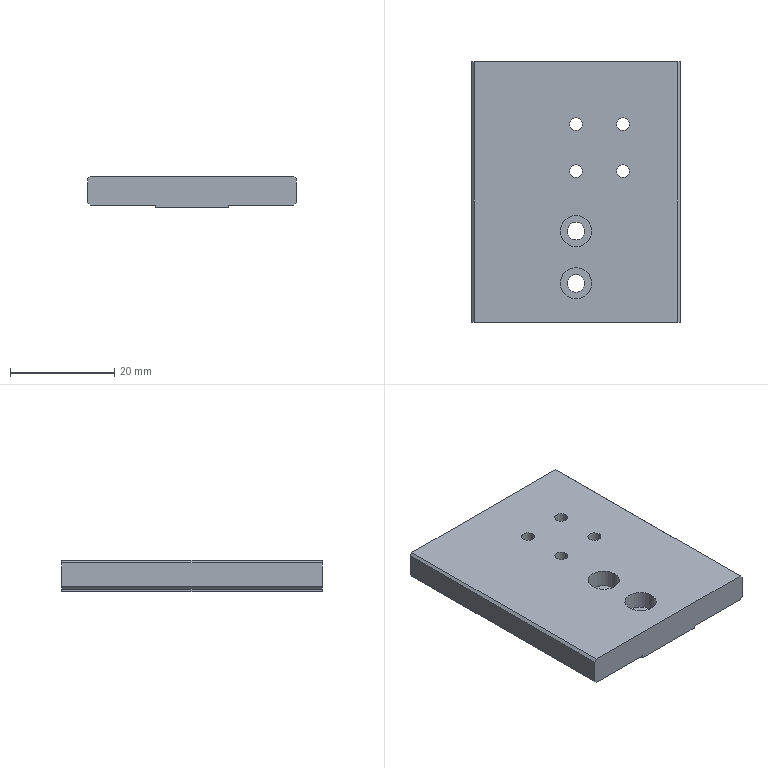Part | SolidWorks | features HoleWzd 2, Chamfer 1, Extrusion 1 | 1 solid | 32 faces | box 40 x 50 x 6 mm | volume 10973 mm3 | cylinder 16 | plane 16 | commonest cylinder face diameters 2.5 x8 3.4 x4 6 x4
STEP:
#1=CARTESIAN_POINT('',(18.75,13.,-6.));
#2=VERTEX_POINT('',#1);
#3=CARTESIAN_POINT('',(21.25,13.,-6.));
#4=VERTEX_POINT('',#3);
#5=CARTESIAN_POINT('',(20.,13.,-6.));
#6=DIRECTION('',(0.,0.,1.));
#7=DIRECTION('',(1.,0.,0.));
#8=AXIS2_PLACEMENT_3D('',#5,#6,#7);
#9=CIRCLE('',#8,1.25);
#10=EDGE_CURVE('',#2,#4,#9,.T.);
#11=ORIENTED_EDGE('',*,*,#10,.F.);
#12=CARTESIAN_POINT('',(18.75,13.,0.));
#13=VERTEX_POINT('',#12);
#14=CARTESIAN_POINT('',(18.75,13.,0.));
#15=DIRECTION('',(0.,0.,1.));
#16=VECTOR('',#15,1000.);
#17=LINE('',#14,#16);
#18=EDGE_CURVE('',#2,#13,#17,.T.);
#19=ORIENTED_EDGE('',*,*,#18,.T.);
#20=CARTESIAN_POINT('',(21.25,13.,0.));
#21=VERTEX_POINT('',#20);
#22=CARTESIAN_POINT('',(20.,13.,0.));
#23=DIRECTION('',(0.,0.,1.));
#24=DIRECTION('',(1.,0.,0.));
#25=AXIS2_PLACEMENT_3D('',#22,#23,#24);
#26=CIRCLE('',#25,1.25);
#27=EDGE_CURVE('',#13,#21,#26,.T.);
#28=ORIENTED_EDGE('',*,*,#27,.T.);
#29=CARTESIAN_POINT('',(21.25,13.,0.));
#30=DIRECTION('',(0.,0.,1.));
#31=VECTOR('',#30,1000.);
#32=LINE('',#29,#31);
#33=EDGE_CURVE('',#4,#21,#32,.T.);
#34=ORIENTED_EDGE('',*,*,#33,.F.);
#35=EDGE_LOOP('',(#11,#19,#28,#34));
#36=FACE_OUTER_BOUND('',#35,.T.);
#37=CARTESIAN_POINT('',(20.,13.,0.));
#38=DIRECTION('',(0.,0.,1.));
#39=DIRECTION('',(1.,0.,0.));
#40=AXIS2_PLACEMENT_3D('',#37,#38,#39);
#41=CYLINDRICAL_SURFACE('',#40,1.25);
#42=ADVANCED_FACE('',(#36),#41,.F.);
#43=CARTESIAN_POINT('',(27.75,13.,-5.5));
#44=VERTEX_POINT('',#43);
#45=CARTESIAN_POINT('',(30.25,13.,-5.5));
#46=VERTEX_POINT('',#45);
#47=CARTESIAN_POINT('',(29.,13.,-5.5));
#48=DIRECTION('',(0.,0.,1.));
#49=DIRECTION('',(1.,0.,0.));
#50=AXIS2_PLACEMENT_3D('',#47,#48,#49);
#51=CIRCLE('',#50,1.25);
#52=EDGE_CURVE('',#44,#46,#51,.T.);
#53=ORIENTED_EDGE('',*,*,#52,.F.);
#54=CARTESIAN_POINT('',(27.75,13.,0.));
#55=VERTEX_POINT('',#54);
#56=CARTESIAN_POINT('',(27.75,13.,0.));
#57=DIRECTION('',(0.,0.,1.));
#58=VECTOR('',#57,1000.);
#59=LINE('',#56,#58);
#60=EDGE_CURVE('',#44,#55,#59,.T.);
#61=ORIENTED_EDGE('',*,*,#60,.T.);
#62=CARTESIAN_POINT('',(30.25,13.,0.));
#63=VERTEX_POINT('',#62);
#64=CARTESIAN_POINT('',(29.,13.,0.));
#65=DIRECTION('',(0.,0.,1.));
#66=DIRECTION('',(1.,0.,0.));
#67=AXIS2_PLACEMENT_3D('',#64,#65,#66);
#68=CIRCLE('',#67,1.25);
#69=EDGE_CURVE('',#55,#63,#68,.T.);
#70=ORIENTED_EDGE('',*,*,#69,.T.);
#71=CARTESIAN_POINT('',(30.25,13.,0.));
#72=DIRECTION('',(0.,0.,1.));
#73=VECTOR('',#72,1000.);
#74=LINE('',#71,#73);
#75=EDGE_CURVE('',#46,#63,#74,.T.);
#76=ORIENTED_EDGE('',*,*,#75,.F.);
#77=EDGE_LOOP('',(#53,#61,#70,#76));
#78=FACE_OUTER_BOUND('',#77,.T.);
#79=CARTESIAN_POINT('',(29.,13.,0.));
#80=DIRECTION('',(0.,0.,1.));
#81=DIRECTION('',(1.,0.,0.));
#82=AXIS2_PLACEMENT_3D('',#79,#80,#81);
#83=CYLINDRICAL_SURFACE('',#82,1.25);
#84=ADVANCED_FACE('',(#78),#83,.F.);
#85=CARTESIAN_POINT('',(18.75,4.,-6.));
#86=VERTEX_POINT('',#85);
#87=CARTESIAN_POINT('',(21.25,4.,-6.));
#88=VERTEX_POINT('',#87);
#89=CARTESIAN_POINT('',(20.,4.,-6.));
#90=DIRECTION('',(0.,0.,1.));
#91=DIRECTION('',(1.,0.,0.));
#92=AXIS2_PLACEMENT_3D('',#89,#90,#91);
#93=CIRCLE('',#92,1.25);
#94=EDGE_CURVE('',#86,#88,#93,.T.);
#95=ORIENTED_EDGE('',*,*,#94,.F.);
#96=CARTESIAN_POINT('',(18.75,4.,0.));
#97=VERTEX_POINT('',#96);
#98=CARTESIAN_POINT('',(18.75,4.,0.));
#99=DIRECTION('',(0.,0.,1.));
#100=VECTOR('',#99,1000.);
#101=LINE('',#98,#100);
#102=EDGE_CURVE('',#86,#97,#101,.T.);
#103=ORIENTED_EDGE('',*,*,#102,.T.);
#104=CARTESIAN_POINT('',(21.25,4.,0.));
#105=VERTEX_POINT('',#104);
#106=CARTESIAN_POINT('',(20.,4.,0.));
#107=DIRECTION('',(0.,0.,1.));
#108=DIRECTION('',(1.,0.,0.));
#109=AXIS2_PLACEMENT_3D('',#106,#107,#108);
#110=CIRCLE('',#109,1.25);
#111=EDGE_CURVE('',#97,#105,#110,.T.);
#112=ORIENTED_EDGE('',*,*,#111,.T.);
#113=CARTESIAN_POINT('',(21.25,4.,0.));
#114=DIRECTION('',(0.,0.,1.));
#115=VECTOR('',#114,1000.);
#116=LINE('',#113,#115);
#117=EDGE_CURVE('',#88,#105,#116,.T.);
#118=ORIENTED_EDGE('',*,*,#117,.F.);
#119=EDGE_LOOP('',(#95,#103,#112,#118));
#120=FACE_OUTER_BOUND('',#119,.T.);
#121=CARTESIAN_POINT('',(20.,4.,0.));
#122=DIRECTION('',(0.,0.,1.));
#123=DIRECTION('',(1.,0.,0.));
#124=AXIS2_PLACEMENT_3D('',#121,#122,#123);
#125=CYLINDRICAL_SURFACE('',#124,1.25);
#126=ADVANCED_FACE('',(#120),#125,.F.);
#127=CARTESIAN_POINT('',(27.75,4.,-5.5));
#128=VERTEX_POINT('',#127);
#129=CARTESIAN_POINT('',(30.25,4.,-5.5));
#130=VERTEX_POINT('',#129);
#131=CARTESIAN_POINT('',(29.,4.,-5.5));
#132=DIRECTION('',(0.,0.,1.));
#133=DIRECTION('',(1.,0.,0.));
#134=AXIS2_PLACEMENT_3D('',#131,#132,#133);
#135=CIRCLE('',#134,1.25);
#136=EDGE_CURVE('',#128,#130,#135,.T.);
#137=ORIENTED_EDGE('',*,*,#136,.F.);
#138=CARTESIAN_POINT('',(27.75,4.,0.));
#139=VERTEX_POINT('',#138);
#140=CARTESIAN_POINT('',(27.75,4.,0.));
#141=DIRECTION('',(0.,0.,1.));
#142=VECTOR('',#141,1000.);
#143=LINE('',#140,#142);
#144=EDGE_CURVE('',#128,#139,#143,.T.);
#145=ORIENTED_EDGE('',*,*,#144,.T.);
#146=CARTESIAN_POINT('',(30.25,4.,0.));
#147=VERTEX_POINT('',#146);
#148=CARTESIAN_POINT('',(29.,4.,0.));
#149=DIRECTION('',(0.,0.,1.));
#150=DIRECTION('',(1.,0.,0.));
#151=AXIS2_PLACEMENT_3D('',#148,#149,#150);
#152=CIRCLE('',#151,1.25);
#153=EDGE_CURVE('',#139,#147,#152,.T.);
#154=ORIENTED_EDGE('',*,*,#153,.T.);
#155=CARTESIAN_POINT('',(30.25,4.,0.));
#156=DIRECTION('',(0.,0.,1.));
#157=VECTOR('',#156,1000.);
#158=LINE('',#155,#157);
#159=EDGE_CURVE('',#130,#147,#158,.T.);
#160=ORIENTED_EDGE('',*,*,#159,.F.);
#161=EDGE_LOOP('',(#137,#145,#154,#160));
#162=FACE_OUTER_BOUND('',#161,.T.);
#163=CARTESIAN_POINT('',(29.,4.,0.));
#164=DIRECTION('',(0.,0.,1.));
#165=DIRECTION('',(1.,0.,0.));
#166=AXIS2_PLACEMENT_3D('',#163,#164,#165);
#167=CYLINDRICAL_SURFACE('',#166,1.25);
#168=ADVANCED_FACE('',(#162),#167,.F.);
#169=CARTESIAN_POINT('',(17.,-7.5,-3.4));
#170=VERTEX_POINT('',#169);
#171=CARTESIAN_POINT('',(23.,-7.5,-3.4));
#172=VERTEX_POINT('',#171);
#173=CARTESIAN_POINT('',(20.,-7.5,-3.4));
#174=DIRECTION('',(0.,0.,1.));
#175=DIRECTION('',(1.,0.,0.));
#176=AXIS2_PLACEMENT_3D('',#173,#174,#175);
#177=CIRCLE('',#176,3.);
#178=EDGE_CURVE('',#170,#172,#177,.T.);
#179=ORIENTED_EDGE('',*,*,#178,.F.);
#180=CARTESIAN_POINT('',(17.,-7.5,0.));
#181=VERTEX_POINT('',#180);
#182=CARTESIAN_POINT('',(17.,-7.5,0.));
#183=DIRECTION('',(0.,0.,1.));
#184=VECTOR('',#183,1000.);
#185=LINE('',#182,#184);
#186=EDGE_CURVE('',#170,#181,#185,.T.);
#187=ORIENTED_EDGE('',*,*,#186,.T.);
#188=CARTESIAN_POINT('',(23.,-7.5,0.));
#189=VERTEX_POINT('',#188);
#190=CARTESIAN_POINT('',(20.,-7.5,0.));
#191=DIRECTION('',(0.,0.,1.));
#192=DIRECTION('',(1.,0.,0.));
#193=AXIS2_PLACEMENT_3D('',#190,#191,#192);
#194=CIRCLE('',#193,3.);
#195=EDGE_CURVE('',#181,#189,#194,.T.);
#196=ORIENTED_EDGE('',*,*,#195,.T.);
#197=CARTESIAN_POINT('',(23.,-7.5,0.));
#198=DIRECTION('',(0.,0.,1.));
#199=VECTOR('',#198,1000.);
#200=LINE('',#197,#199);
#201=EDGE_CURVE('',#172,#189,#200,.T.);
#202=ORIENTED_EDGE('',*,*,#201,.F.);
#203=EDGE_LOOP('',(#179,#187,#196,#202));
#204=FACE_OUTER_BOUND('',#203,.T.);
#205=CARTESIAN_POINT('',(20.,-7.5,0.));
#206=DIRECTION('',(0.,0.,1.));
#207=DIRECTION('',(1.,0.,0.));
#208=AXIS2_PLACEMENT_3D('',#205,#206,#207);
#209=CYLINDRICAL_SURFACE('',#208,3.);
#210=ADVANCED_FACE('',(#204),#209,.F.);
#211=CARTESIAN_POINT('',(18.3,-7.5,-6.));
#212=VERTEX_POINT('',#211);
#213=CARTESIAN_POINT('',(21.7,-7.5,-6.));
#214=VERTEX_POINT('',#213);
#215=CARTESIAN_POINT('',(20.,-7.5,-6.));
#216=DIRECTION('',(0.,0.,1.));
#217=DIRECTION('',(1.,0.,0.));
#218=AXIS2_PLACEMENT_3D('',#215,#216,#217);
#219=CIRCLE('',#218,1.7);
#220=EDGE_CURVE('',#212,#214,#219,.T.);
#221=ORIENTED_EDGE('',*,*,#220,.F.);
#222=CARTESIAN_POINT('',(18.3,-7.5,-3.4));
#223=VERTEX_POINT('',#222);
#224=CARTESIAN_POINT('',(18.3,-7.5,0.));
#225=DIRECTION('',(0.,0.,1.));
#226=VECTOR('',#225,1000.);
#227=LINE('',#224,#226);
#228=EDGE_CURVE('',#212,#223,#227,.T.);
#229=ORIENTED_EDGE('',*,*,#228,.T.);
#230=CARTESIAN_POINT('',(21.7,-7.5,-3.4));
#231=VERTEX_POINT('',#230);
#232=CARTESIAN_POINT('',(20.,-7.5,-3.4));
#233=DIRECTION('',(0.,0.,1.));
#234=DIRECTION('',(1.,0.,0.));
#235=AXIS2_PLACEMENT_3D('',#232,#233,#234);
#236=CIRCLE('',#235,1.7);
#237=EDGE_CURVE('',#223,#231,#236,.T.);
#238=ORIENTED_EDGE('',*,*,#237,.T.);
#239=CARTESIAN_POINT('',(21.7,-7.5,0.));
#240=DIRECTION('',(0.,0.,1.));
#241=VECTOR('',#240,1000.);
#242=LINE('',#239,#241);
#243=EDGE_CURVE('',#214,#231,#242,.T.);
#244=ORIENTED_EDGE('',*,*,#243,.F.);
#245=EDGE_LOOP('',(#221,#229,#238,#244));
#246=FACE_OUTER_BOUND('',#245,.T.);
#247=CARTESIAN_POINT('',(20.,-7.5,0.));
#248=DIRECTION('',(0.,0.,1.));
#249=DIRECTION('',(1.,0.,0.));
#250=AXIS2_PLACEMENT_3D('',#247,#248,#249);
#251=CYLINDRICAL_SURFACE('',#250,1.7);
#252=ADVANCED_FACE('',(#246),#251,.F.);
#253=CARTESIAN_POINT('',(17.,-17.5,-3.4));
#254=VERTEX_POINT('',#253);
#255=CARTESIAN_POINT('',(23.,-17.5,-3.4));
#256=VERTEX_POINT('',#255);
#257=CARTESIAN_POINT('',(20.,-17.5,-3.4));
#258=DIRECTION('',(0.,0.,1.));
#259=DIRECTION('',(1.,0.,0.));
#260=AXIS2_PLACEMENT_3D('',#257,#258,#259);
#261=CIRCLE('',#260,3.);
#262=EDGE_CURVE('',#254,#256,#261,.T.);
#263=ORIENTED_EDGE('',*,*,#262,.F.);
#264=CARTESIAN_POINT('',(17.,-17.5,0.));
#265=VERTEX_POINT('',#264);
#266=CARTESIAN_POINT('',(17.,-17.5,0.));
#267=DIRECTION('',(0.,0.,1.));
#268=VECTOR('',#267,1000.);
#269=LINE('',#266,#268);
#270=EDGE_CURVE('',#254,#265,#269,.T.);
#271=ORIENTED_EDGE('',*,*,#270,.T.);
#272=CARTESIAN_POINT('',(23.,-17.5,0.));
#273=VERTEX_POINT('',#272);
#274=CARTESIAN_POINT('',(20.,-17.5,0.));
#275=DIRECTION('',(0.,0.,1.));
#276=DIRECTION('',(1.,0.,0.));
#277=AXIS2_PLACEMENT_3D('',#274,#275,#276);
#278=CIRCLE('',#277,3.);
#279=EDGE_CURVE('',#265,#273,#278,.T.);
#280=ORIENTED_EDGE('',*,*,#279,.T.);
#281=CARTESIAN_POINT('',(23.,-17.5,0.));
#282=DIRECTION('',(0.,0.,1.));
#283=VECTOR('',#282,1000.);
#284=LINE('',#281,#283);
#285=EDGE_CURVE('',#256,#273,#284,.T.);
#286=ORIENTED_EDGE('',*,*,#285,.F.);
#287=EDGE_LOOP('',(#263,#271,#280,#286));
#288=FACE_OUTER_BOUND('',#287,.T.);
#289=CARTESIAN_POINT('',(20.,-17.5,0.));
#290=DIRECTION('',(0.,0.,1.));
#291=DIRECTION('',(1.,0.,0.));
#292=AXIS2_PLACEMENT_3D('',#289,#290,#291);
#293=CYLINDRICAL_SURFACE('',#292,3.);
#294=ADVANCED_FACE('',(#288),#293,.F.);
#295=CARTESIAN_POINT('',(18.3,-17.5,-6.));
#296=VERTEX_POINT('',#295);
#297=CARTESIAN_POINT('',(21.7,-17.5,-6.));
#298=VERTEX_POINT('',#297);
#299=CARTESIAN_POINT('',(20.,-17.5,-6.));
#300=DIRECTION('',(0.,0.,1.));
#301=DIRECTION('',(1.,0.,0.));
#302=AXIS2_PLACEMENT_3D('',#299,#300,#301);
#303=CIRCLE('',#302,1.7);
#304=EDGE_CURVE('',#296,#298,#303,.T.);
#305=ORIENTED_EDGE('',*,*,#304,.F.);
#306=CARTESIAN_POINT('',(18.3,-17.5,-3.4));
#307=VERTEX_POINT('',#306);
#308=CARTESIAN_POINT('',(18.3,-17.5,0.));
#309=DIRECTION('',(0.,0.,1.));
#310=VECTOR('',#309,1000.);
#311=LINE('',#308,#310);
#312=EDGE_CURVE('',#296,#307,#311,.T.);
#313=ORIENTED_EDGE('',*,*,#312,.T.);
#314=CARTESIAN_POINT('',(21.7,-17.5,-3.4));
#315=VERTEX_POINT('',#314);
#316=CARTESIAN_POINT('',(20.,-17.5,-3.4));
#317=DIRECTION('',(0.,0.,1.));
#318=DIRECTION('',(1.,0.,0.));
#319=AXIS2_PLACEMENT_3D('',#316,#317,#318);
#320=CIRCLE('',#319,1.7);
#321=EDGE_CURVE('',#307,#315,#320,.T.);
#322=ORIENTED_EDGE('',*,*,#321,.T.);
#323=CARTESIAN_POINT('',(21.7,-17.5,0.));
#324=DIRECTION('',(0.,0.,1.));
#325=VECTOR('',#324,1000.);
#326=LINE('',#323,#325);
#327=EDGE_CURVE('',#298,#315,#326,.T.);
#328=ORIENTED_EDGE('',*,*,#327,.F.);
#329=EDGE_LOOP('',(#305,#313,#322,#328));
#330=FACE_OUTER_BOUND('',#329,.T.);
#331=CARTESIAN_POINT('',(20.,-17.5,0.));
#332=DIRECTION('',(0.,0.,1.));
#333=DIRECTION('',(1.,0.,0.));
#334=AXIS2_PLACEMENT_3D('',#331,#332,#333);
#335=CYLINDRICAL_SURFACE('',#334,1.7);
#336=ADVANCED_FACE('',(#330),#335,.F.);
#337=CARTESIAN_POINT('',(0.,-25.,-5.));
#338=VERTEX_POINT('',#337);
#339=CARTESIAN_POINT('',(0.,-25.,-0.5));
#340=VERTEX_POINT('',#339);
#341=CARTESIAN_POINT('',(0.,-25.,-5.5));
#342=DIRECTION('',(0.,0.,1.));
#343=VECTOR('',#342,1000.);
#344=LINE('',#341,#343);
#345=EDGE_CURVE('',#338,#340,#344,.T.);
#346=ORIENTED_EDGE('',*,*,#345,.T.);
#347=CARTESIAN_POINT('',(0.,25.,-0.5));
#348=VERTEX_POINT('',#347);
#349=CARTESIAN_POINT('',(0.,25.,-0.5));
#350=DIRECTION('',(0.,1.,0.));
#351=VECTOR('',#350,1000.);
#352=LINE('',#349,#351);
#353=EDGE_CURVE('',#340,#348,#352,.T.);
#354=ORIENTED_EDGE('',*,*,#353,.T.);
#355=CARTESIAN_POINT('',(0.,25.,-5.));
#356=VERTEX_POINT('',#355);
#357=CARTESIAN_POINT('',(0.,25.,-5.5));
#358=DIRECTION('',(0.,0.,1.));
#359=VECTOR('',#358,1000.);
#360=LINE('',#357,#359);
#361=EDGE_CURVE('',#356,#348,#360,.T.);
#362=ORIENTED_EDGE('',*,*,#361,.F.);
#363=CARTESIAN_POINT('',(0.,25.,-5.));
#364=DIRECTION('',(0.,-1.,0.));
#365=VECTOR('',#364,1000.);
#366=LINE('',#363,#365);
#367=EDGE_CURVE('',#356,#338,#366,.T.);
#368=ORIENTED_EDGE('',*,*,#367,.T.);
#369=EDGE_LOOP('',(#346,#354,#362,#368));
#370=FACE_OUTER_BOUND('',#369,.T.);
#371=CARTESIAN_POINT('',(0.,25.,-5.5));
#372=DIRECTION('',(1.,0.,0.));
#373=DIRECTION('',(0.,0.,-1.));
#374=AXIS2_PLACEMENT_3D('',#371,#372,#373);
#375=PLANE('',#374);
#376=ADVANCED_FACE('',(#370),#375,.F.);
#377=CARTESIAN_POINT('',(20.,13.,0.));
#378=DIRECTION('',(0.,0.,1.));
#379=DIRECTION('',(1.,0.,0.));
#380=AXIS2_PLACEMENT_3D('',#377,#378,#379);
#381=CIRCLE('',#380,1.25);
#382=EDGE_CURVE('',#21,#13,#381,.T.);
#383=ORIENTED_EDGE('',*,*,#382,.F.);
#384=ORIENTED_EDGE('',*,*,#27,.F.);
#385=EDGE_LOOP('',(#383,#384));
#386=FACE_BOUND('',#385,.T.);
#387=CARTESIAN_POINT('',(29.,13.,0.));
#388=DIRECTION('',(0.,0.,1.));
#389=DIRECTION('',(1.,0.,0.));
#390=AXIS2_PLACEMENT_3D('',#387,#388,#389);
#391=CIRCLE('',#390,1.25);
#392=EDGE_CURVE('',#63,#55,#391,.T.);
#393=ORIENTED_EDGE('',*,*,#392,.F.);
#394=ORIENTED_EDGE('',*,*,#69,.F.);
#395=EDGE_LOOP('',(#393,#394));
#396=FACE_BOUND('',#395,.T.);
#397=CARTESIAN_POINT('',(20.,4.,0.));
#398=DIRECTION('',(0.,0.,1.));
#399=DIRECTION('',(1.,0.,0.));
#400=AXIS2_PLACEMENT_3D('',#397,#398,#399);
#401=CIRCLE('',#400,1.25);
#402=EDGE_CURVE('',#105,#97,#401,.T.);
#403=ORIENTED_EDGE('',*,*,#402,.F.);
#404=ORIENTED_EDGE('',*,*,#111,.F.);
#405=EDGE_LOOP('',(#403,#404));
#406=FACE_BOUND('',#405,.T.);
#407=CARTESIAN_POINT('',(29.,4.,0.));
#408=DIRECTION('',(0.,0.,1.));
#409=DIRECTION('',(1.,0.,0.));
#410=AXIS2_PLACEMENT_3D('',#407,#408,#409);
#411=CIRCLE('',#410,1.25);
#412=EDGE_CURVE('',#147,#139,#411,.T.);
#413=ORIENTED_EDGE('',*,*,#412,.F.);
#414=ORIENTED_EDGE('',*,*,#153,.F.);
#415=EDGE_LOOP('',(#413,#414));
#416=FACE_BOUND('',#415,.T.);
#417=CARTESIAN_POINT('',(20.,-7.5,0.));
#418=DIRECTION('',(0.,0.,1.));
#419=DIRECTION('',(1.,0.,0.));
#420=AXIS2_PLACEMENT_3D('',#417,#418,#419);
#421=CIRCLE('',#420,3.);
#422=EDGE_CURVE('',#189,#181,#421,.T.);
#423=ORIENTED_EDGE('',*,*,#422,.F.);
#424=ORIENTED_EDGE('',*,*,#195,.F.);
#425=EDGE_LOOP('',(#423,#424));
#426=FACE_BOUND('',#425,.T.);
#427=CARTESIAN_POINT('',(20.,-17.5,0.));
#428=DIRECTION('',(0.,0.,1.));
#429=DIRECTION('',(1.,0.,0.));
#430=AXIS2_PLACEMENT_3D('',#427,#428,#429);
#431=CIRCLE('',#430,3.);
#432=EDGE_CURVE('',#273,#265,#431,.T.);
#433=ORIENTED_EDGE('',*,*,#432,.F.);
#434=ORIENTED_EDGE('',*,*,#279,.F.);
#435=EDGE_LOOP('',(#433,#434));
#436=FACE_BOUND('',#435,.T.);
#437=CARTESIAN_POINT('',(0.5,-25.,0.));
#438=VERTEX_POINT('',#437);
#439=CARTESIAN_POINT('',(39.5,-25.,0.));
#440=VERTEX_POINT('',#439);
#441=CARTESIAN_POINT('',(0.,-25.,0.));
#442=DIRECTION('',(1.,0.,0.));
#443=VECTOR('',#442,1000.);
#444=LINE('',#441,#443);
#445=EDGE_CURVE('',#438,#440,#444,.T.);
#446=ORIENTED_EDGE('',*,*,#445,.T.);
#447=CARTESIAN_POINT('',(39.5,25.,0.));
#448=VERTEX_POINT('',#447);
#449=CARTESIAN_POINT('',(39.5,25.,0.));
#450=DIRECTION('',(0.,1.,0.));
#451=VECTOR('',#450,1000.);
#452=LINE('',#449,#451);
#453=EDGE_CURVE('',#440,#448,#452,.T.);
#454=ORIENTED_EDGE('',*,*,#453,.T.);
#455=CARTESIAN_POINT('',(0.5,25.,0.));
#456=VERTEX_POINT('',#455);
#457=CARTESIAN_POINT('',(0.,25.,0.));
#458=DIRECTION('',(1.,0.,0.));
#459=VECTOR('',#458,1000.);
#460=LINE('',#457,#459);
#461=EDGE_CURVE('',#456,#448,#460,.T.);
#462=ORIENTED_EDGE('',*,*,#461,.F.);
#463=CARTESIAN_POINT('',(0.5,25.,0.));
#464=DIRECTION('',(0.,-1.,0.));
#465=VECTOR('',#464,1000.);
#466=LINE('',#463,#465);
#467=EDGE_CURVE('',#456,#438,#466,.T.);
#468=ORIENTED_EDGE('',*,*,#467,.T.);
#469=EDGE_LOOP('',(#446,#454,#462,#468));
#470=FACE_OUTER_BOUND('',#469,.T.);
#471=CARTESIAN_POINT('',(0.,25.,0.));
#472=DIRECTION('',(0.,0.,-1.));
#473=DIRECTION('',(-1.,0.,0.));
#474=AXIS2_PLACEMENT_3D('',#471,#472,#473);
#475=PLANE('',#474);
#476=ADVANCED_FACE('',(#386,#396,#406,#416,#426,#436,#470),#475,.F.);
#477=CARTESIAN_POINT('',(40.,-25.,-0.5));
#478=VERTEX_POINT('',#477);
#479=CARTESIAN_POINT('',(40.,-25.,-5.));
#480=VERTEX_POINT('',#479);
#481=CARTESIAN_POINT('',(40.,-25.,0.));
#482=DIRECTION('',(0.,0.,-1.));
#483=VECTOR('',#482,1000.);
#484=LINE('',#481,#483);
#485=EDGE_CURVE('',#478,#480,#484,.T.);
#486=ORIENTED_EDGE('',*,*,#485,.T.);
#487=CARTESIAN_POINT('',(40.,25.,-5.));
#488=VERTEX_POINT('',#487);
#489=CARTESIAN_POINT('',(40.,25.,-5.));
#490=DIRECTION('',(0.,1.,0.));
#491=VECTOR('',#490,1000.);
#492=LINE('',#489,#491);
#493=EDGE_CURVE('',#480,#488,#492,.T.);
#494=ORIENTED_EDGE('',*,*,#493,.T.);
#495=CARTESIAN_POINT('',(40.,25.,-0.5));
#496=VERTEX_POINT('',#495);
#497=CARTESIAN_POINT('',(40.,25.,0.));
#498=DIRECTION('',(0.,0.,-1.));
#499=VECTOR('',#498,1000.);
#500=LINE('',#497,#499);
#501=EDGE_CURVE('',#496,#488,#500,.T.);
#502=ORIENTED_EDGE('',*,*,#501,.F.);
#503=CARTESIAN_POINT('',(40.,25.,-0.5));
#504=DIRECTION('',(0.,-1.,0.));
#505=VECTOR('',#504,1000.);
#506=LINE('',#503,#505);
#507=EDGE_CURVE('',#496,#478,#506,.T.);
#508=ORIENTED_EDGE('',*,*,#507,.T.);
#509=EDGE_LOOP('',(#486,#494,#502,#508));
#510=FACE_OUTER_BOUND('',#509,.T.);
#511=CARTESIAN_POINT('',(40.,25.,0.));
#512=DIRECTION('',(-1.,0.,0.));
#513=DIRECTION('',(0.,0.,1.));
#514=AXIS2_PLACEMENT_3D('',#511,#512,#513);
#515=PLANE('',#514);
#516=ADVANCED_FACE('',(#510),#515,.F.);
#517=CARTESIAN_POINT('',(29.,13.,-5.5));
#518=DIRECTION('',(0.,0.,1.));
#519=DIRECTION('',(1.,0.,0.));
#520=AXIS2_PLACEMENT_3D('',#517,#518,#519);
#521=CIRCLE('',#520,1.25);
#522=EDGE_CURVE('',#46,#44,#521,.T.);
#523=ORIENTED_EDGE('',*,*,#522,.T.);
#524=ORIENTED_EDGE('',*,*,#52,.T.);
#525=EDGE_LOOP('',(#523,#524));
#526=FACE_BOUND('',#525,.T.);
#527=CARTESIAN_POINT('',(29.,4.,-5.5));
#528=DIRECTION('',(0.,0.,1.));
#529=DIRECTION('',(1.,0.,0.));
#530=AXIS2_PLACEMENT_3D('',#527,#528,#529);
#531=CIRCLE('',#530,1.25);
#532=EDGE_CURVE('',#130,#128,#531,.T.);
#533=ORIENTED_EDGE('',*,*,#532,.T.);
#534=ORIENTED_EDGE('',*,*,#136,.T.);
#535=EDGE_LOOP('',(#533,#534));
#536=FACE_BOUND('',#535,.T.);
#537=CARTESIAN_POINT('',(39.5,25.,-5.5));
#538=VERTEX_POINT('',#537);
#539=CARTESIAN_POINT('',(27.,25.,-5.5));
#540=VERTEX_POINT('',#539);
#541=CARTESIAN_POINT('',(40.,25.,-5.5));
#542=DIRECTION('',(-1.,0.,0.));
#543=VECTOR('',#542,1000.);
#544=LINE('',#541,#543);
#545=EDGE_CURVE('',#538,#540,#544,.T.);
#546=ORIENTED_EDGE('',*,*,#545,.F.);
#547=CARTESIAN_POINT('',(39.5,-25.,-5.5));
#548=VERTEX_POINT('',#547);
#549=CARTESIAN_POINT('',(39.5,25.,-5.5));
#550=DIRECTION('',(0.,-1.,0.));
#551=VECTOR('',#550,1000.);
#552=LINE('',#549,#551);
#553=EDGE_CURVE('',#538,#548,#552,.T.);
#554=ORIENTED_EDGE('',*,*,#553,.T.);
#555=CARTESIAN_POINT('',(27.,-25.,-5.5));
#556=VERTEX_POINT('',#555);
#557=CARTESIAN_POINT('',(40.,-25.,-5.5));
#558=DIRECTION('',(-1.,0.,0.));
#559=VECTOR('',#558,1000.);
#560=LINE('',#557,#559);
#561=EDGE_CURVE('',#548,#556,#560,.T.);
#562=ORIENTED_EDGE('',*,*,#561,.T.);
#563=CARTESIAN_POINT('',(27.,25.,-5.5));
#564=DIRECTION('',(0.,-1.,0.));
#565=VECTOR('',#564,1000.);
#566=LINE('',#563,#565);
#567=EDGE_CURVE('',#540,#556,#566,.T.);
#568=ORIENTED_EDGE('',*,*,#567,.F.);
#569=EDGE_LOOP('',(#546,#554,#562,#568));
#570=FACE_OUTER_BOUND('',#569,.T.);
#571=CARTESIAN_POINT('',(40.,25.,-5.5));
#572=DIRECTION('',(0.,0.,1.));
#573=DIRECTION('',(1.,0.,0.));
#574=AXIS2_PLACEMENT_3D('',#571,#572,#573);
#575=PLANE('',#574);
#576=ADVANCED_FACE('',(#526,#536,#570),#575,.F.);
#577=CARTESIAN_POINT('',(27.,-25.,-6.));
#578=VERTEX_POINT('',#577);
#579=CARTESIAN_POINT('',(27.,-25.,-5.5));
#580=DIRECTION('',(0.,0.,-1.));
#581=VECTOR('',#580,1000.);
#582=LINE('',#579,#581);
#583=EDGE_CURVE('',#556,#578,#582,.T.);
#584=ORIENTED_EDGE('',*,*,#583,.T.);
#585=CARTESIAN_POINT('',(27.,25.,-6.));
#586=VERTEX_POINT('',#585);
#587=CARTESIAN_POINT('',(27.,25.,-6.));
#588=DIRECTION('',(0.,-1.,0.));
#589=VECTOR('',#588,1000.);
#590=LINE('',#587,#589);
#591=EDGE_CURVE('',#586,#578,#590,.T.);
#592=ORIENTED_EDGE('',*,*,#591,.F.);
#593=CARTESIAN_POINT('',(27.,25.,-5.5));
#594=DIRECTION('',(0.,0.,-1.));
#595=VECTOR('',#594,1000.);
#596=LINE('',#593,#595);
#597=EDGE_CURVE('',#540,#586,#596,.T.);
#598=ORIENTED_EDGE('',*,*,#597,.F.);
#599=ORIENTED_EDGE('',*,*,#567,.T.);
#600=EDGE_LOOP('',(#584,#592,#598,#599));
#601=FACE_OUTER_BOUND('',#600,.T.);
#602=CARTESIAN_POINT('',(27.,25.,-5.5));
#603=DIRECTION('',(-1.,0.,0.));
#604=DIRECTION('',(0.,0.,1.));
#605=AXIS2_PLACEMENT_3D('',#602,#603,#604);
#606=PLANE('',#605);
#607=ADVANCED_FACE('',(#601),#606,.F.);
#608=CARTESIAN_POINT('',(20.,13.,-6.));
#609=DIRECTION('',(0.,0.,1.));
#610=DIRECTION('',(1.,0.,0.));
#611=AXIS2_PLACEMENT_3D('',#608,#609,#610);
#612=CIRCLE('',#611,1.25);
#613=EDGE_CURVE('',#4,#2,#612,.T.);
#614=ORIENTED_EDGE('',*,*,#613,.T.);
#615=ORIENTED_EDGE('',*,*,#10,.T.);
#616=EDGE_LOOP('',(#614,#615));
#617=FACE_BOUND('',#616,.T.);
#618=CARTESIAN_POINT('',(20.,4.,-6.));
#619=DIRECTION('',(0.,0.,1.));
#620=DIRECTION('',(1.,0.,0.));
#621=AXIS2_PLACEMENT_3D('',#618,#619,#620);
#622=CIRCLE('',#621,1.25);
#623=EDGE_CURVE('',#88,#86,#622,.T.);
#624=ORIENTED_EDGE('',*,*,#623,.T.);
#625=ORIENTED_EDGE('',*,*,#94,.T.);
#626=EDGE_LOOP('',(#624,#625));
#627=FACE_BOUND('',#626,.T.);
#628=CARTESIAN_POINT('',(20.,-7.5,-6.));
#629=DIRECTION('',(0.,0.,1.));
#630=DIRECTION('',(1.,0.,0.));
#631=AXIS2_PLACEMENT_3D('',#628,#629,#630);
#632=CIRCLE('',#631,1.7);
#633=EDGE_CURVE('',#214,#212,#632,.T.);
#634=ORIENTED_EDGE('',*,*,#633,.T.);
#635=ORIENTED_EDGE('',*,*,#220,.T.);
#636=EDGE_LOOP('',(#634,#635));
#637=FACE_BOUND('',#636,.T.);
#638=CARTESIAN_POINT('',(20.,-17.5,-6.));
#639=DIRECTION('',(0.,0.,1.));
#640=DIRECTION('',(1.,0.,0.));
#641=AXIS2_PLACEMENT_3D('',#638,#639,#640);
#642=CIRCLE('',#641,1.7);
#643=EDGE_CURVE('',#298,#296,#642,.T.);
#644=ORIENTED_EDGE('',*,*,#643,.T.);
#645=ORIENTED_EDGE('',*,*,#304,.T.);
#646=EDGE_LOOP('',(#644,#645));
#647=FACE_BOUND('',#646,.T.);
#648=CARTESIAN_POINT('',(13.,-25.,-6.));
#649=VERTEX_POINT('',#648);
#650=CARTESIAN_POINT('',(27.,-25.,-6.));
#651=DIRECTION('',(-1.,0.,0.));
#652=VECTOR('',#651,1000.);
#653=LINE('',#650,#652);
#654=EDGE_CURVE('',#578,#649,#653,.T.);
#655=ORIENTED_EDGE('',*,*,#654,.T.);
#656=CARTESIAN_POINT('',(13.,25.,-6.));
#657=VERTEX_POINT('',#656);
#658=CARTESIAN_POINT('',(13.,25.,-6.));
#659=DIRECTION('',(0.,-1.,0.));
#660=VECTOR('',#659,1000.);
#661=LINE('',#658,#660);
#662=EDGE_CURVE('',#657,#649,#661,.T.);
#663=ORIENTED_EDGE('',*,*,#662,.F.);
#664=CARTESIAN_POINT('',(27.,25.,-6.));
#665=DIRECTION('',(-1.,0.,0.));
#666=VECTOR('',#665,1000.);
#667=LINE('',#664,#666);
#668=EDGE_CURVE('',#586,#657,#667,.T.);
#669=ORIENTED_EDGE('',*,*,#668,.F.);
#670=ORIENTED_EDGE('',*,*,#591,.T.);
#671=EDGE_LOOP('',(#655,#663,#669,#670));
#672=FACE_OUTER_BOUND('',#671,.T.);
#673=CARTESIAN_POINT('',(27.,25.,-6.));
#674=DIRECTION('',(0.,0.,1.));
#675=DIRECTION('',(1.,0.,0.));
#676=AXIS2_PLACEMENT_3D('',#673,#674,#675);
#677=PLANE('',#676);
#678=ADVANCED_FACE('',(#617,#627,#637,#647,#672),#677,.F.);
#679=CARTESIAN_POINT('',(13.,-25.,-5.5));
#680=VERTEX_POINT('',#679);
#681=CARTESIAN_POINT('',(13.,-25.,-6.));
#682=DIRECTION('',(0.,0.,1.));
#683=VECTOR('',#682,1000.);
#684=LINE('',#681,#683);
#685=EDGE_CURVE('',#649,#680,#684,.T.);
#686=ORIENTED_EDGE('',*,*,#685,.T.);
#687=CARTESIAN_POINT('',(13.,25.,-5.5));
#688=VERTEX_POINT('',#687);
#689=CARTESIAN_POINT('',(13.,25.,-5.5));
#690=DIRECTION('',(0.,-1.,0.));
#691=VECTOR('',#690,1000.);
#692=LINE('',#689,#691);
#693=EDGE_CURVE('',#688,#680,#692,.T.);
#694=ORIENTED_EDGE('',*,*,#693,.F.);
#695=CARTESIAN_POINT('',(13.,25.,-6.));
#696=DIRECTION('',(0.,0.,1.));
#697=VECTOR('',#696,1000.);
#698=LINE('',#695,#697);
#699=EDGE_CURVE('',#657,#688,#698,.T.);
#700=ORIENTED_EDGE('',*,*,#699,.F.);
#701=ORIENTED_EDGE('',*,*,#662,.T.);
#702=EDGE_LOOP('',(#686,#694,#700,#701));
#703=FACE_OUTER_BOUND('',#702,.T.);
#704=CARTESIAN_POINT('',(13.,25.,-6.));
#705=DIRECTION('',(1.,0.,0.));
#706=DIRECTION('',(0.,0.,-1.));
#707=AXIS2_PLACEMENT_3D('',#704,#705,#706);
#708=PLANE('',#707);
#709=ADVANCED_FACE('',(#703),#708,.F.);
#710=CARTESIAN_POINT('',(0.5,-25.,-5.5));
#711=VERTEX_POINT('',#710);
#712=CARTESIAN_POINT('',(13.,-25.,-5.5));
#713=DIRECTION('',(-1.,0.,0.));
#714=VECTOR('',#713,1000.);
#715=LINE('',#712,#714);
#716=EDGE_CURVE('',#680,#711,#715,.T.);
#717=ORIENTED_EDGE('',*,*,#716,.T.);
#718=CARTESIAN_POINT('',(0.5,25.,-5.5));
#719=VERTEX_POINT('',#718);
#720=CARTESIAN_POINT('',(0.5,25.,-5.5));
#721=DIRECTION('',(0.,1.,0.));
#722=VECTOR('',#721,1000.);
#723=LINE('',#720,#722);
#724=EDGE_CURVE('',#711,#719,#723,.T.);
#725=ORIENTED_EDGE('',*,*,#724,.T.);
#726=CARTESIAN_POINT('',(13.,25.,-5.5));
#727=DIRECTION('',(-1.,0.,0.));
#728=VECTOR('',#727,1000.);
#729=LINE('',#726,#728);
#730=EDGE_CURVE('',#688,#719,#729,.T.);
#731=ORIENTED_EDGE('',*,*,#730,.F.);
#732=ORIENTED_EDGE('',*,*,#693,.T.);
#733=EDGE_LOOP('',(#717,#725,#731,#732));
#734=FACE_OUTER_BOUND('',#733,.T.);
#735=CARTESIAN_POINT('',(13.,25.,-5.5));
#736=DIRECTION('',(0.,0.,1.));
#737=DIRECTION('',(1.,0.,0.));
#738=AXIS2_PLACEMENT_3D('',#735,#736,#737);
#739=PLANE('',#738);
#740=ADVANCED_FACE('',(#734),#739,.F.);
#741=ORIENTED_EDGE('',*,*,#501,.T.);
#742=CARTESIAN_POINT('',(22.5,25.,-22.5));
#743=DIRECTION('',(-0.7071,0.,-0.7071));
#744=VECTOR('',#743,1000.);
#745=LINE('',#742,#744);
#746=EDGE_CURVE('',#488,#538,#745,.T.);
#747=ORIENTED_EDGE('',*,*,#746,.T.);
#748=ORIENTED_EDGE('',*,*,#545,.T.);
#749=ORIENTED_EDGE('',*,*,#597,.T.);
#750=ORIENTED_EDGE('',*,*,#668,.T.);
#751=ORIENTED_EDGE('',*,*,#699,.T.);
#752=ORIENTED_EDGE('',*,*,#730,.T.);
#753=CARTESIAN_POINT('',(-2.5,25.,-2.5));
#754=DIRECTION('',(-0.7071,0.,0.7071));
#755=VECTOR('',#754,1000.);
#756=LINE('',#753,#755);
#757=EDGE_CURVE('',#719,#356,#756,.T.);
#758=ORIENTED_EDGE('',*,*,#757,.T.);
#759=ORIENTED_EDGE('',*,*,#361,.T.);
#760=CARTESIAN_POINT('',(0.25,25.,-0.25));
#761=DIRECTION('',(0.7071,0.,0.7071));
#762=VECTOR('',#761,1000.);
#763=LINE('',#760,#762);
#764=EDGE_CURVE('',#348,#456,#763,.T.);
#765=ORIENTED_EDGE('',*,*,#764,.T.);
#766=ORIENTED_EDGE('',*,*,#461,.T.);
#767=CARTESIAN_POINT('',(19.75,25.,19.75));
#768=DIRECTION('',(0.7071,0.,-0.7071));
#769=VECTOR('',#768,1000.);
#770=LINE('',#767,#769);
#771=EDGE_CURVE('',#448,#496,#770,.T.);
#772=ORIENTED_EDGE('',*,*,#771,.T.);
#773=EDGE_LOOP('',(#741,#747,#748,#749,#750,#751,#752,#758,#759,#765,#766,#772));
#774=FACE_OUTER_BOUND('',#773,.T.);
#775=CARTESIAN_POINT('',(0.,25.,0.));
#776=DIRECTION('',(0.,1.,0.));
#777=DIRECTION('',(0.,0.,1.));
#778=AXIS2_PLACEMENT_3D('',#775,#776,#777);
#779=PLANE('',#778);
#780=ADVANCED_FACE('',(#774),#779,.T.);
#781=ORIENTED_EDGE('',*,*,#561,.F.);
#782=CARTESIAN_POINT('',(39.5,-25.,-5.5));
#783=DIRECTION('',(0.7071,0.,0.7071));
#784=VECTOR('',#783,1000.);
#785=LINE('',#782,#784);
#786=EDGE_CURVE('',#548,#480,#785,.T.);
#787=ORIENTED_EDGE('',*,*,#786,.T.);
#788=ORIENTED_EDGE('',*,*,#485,.F.);
#789=CARTESIAN_POINT('',(40.,-25.,-0.5));
#790=DIRECTION('',(-0.7071,0.,0.7071));
#791=VECTOR('',#790,1000.);
#792=LINE('',#789,#791);
#793=EDGE_CURVE('',#478,#440,#792,.T.);
#794=ORIENTED_EDGE('',*,*,#793,.T.);
#795=ORIENTED_EDGE('',*,*,#445,.F.);
#796=CARTESIAN_POINT('',(0.5,-25.,0.));
#797=DIRECTION('',(-0.7071,0.,-0.7071));
#798=VECTOR('',#797,1000.);
#799=LINE('',#796,#798);
#800=EDGE_CURVE('',#438,#340,#799,.T.);
#801=ORIENTED_EDGE('',*,*,#800,.T.);
#802=ORIENTED_EDGE('',*,*,#345,.F.);
#803=CARTESIAN_POINT('',(0.,-25.,-5.));
#804=DIRECTION('',(0.7071,0.,-0.7071));
#805=VECTOR('',#804,1000.);
#806=LINE('',#803,#805);
#807=EDGE_CURVE('',#338,#711,#806,.T.);
#808=ORIENTED_EDGE('',*,*,#807,.T.);
#809=ORIENTED_EDGE('',*,*,#716,.F.);
#810=ORIENTED_EDGE('',*,*,#685,.F.);
#811=ORIENTED_EDGE('',*,*,#654,.F.);
#812=ORIENTED_EDGE('',*,*,#583,.F.);
#813=EDGE_LOOP('',(#781,#787,#788,#794,#795,#801,#802,#808,#809,#810,#811,#812));
#814=FACE_OUTER_BOUND('',#813,.T.);
#815=CARTESIAN_POINT('',(0.,-25.,0.));
#816=DIRECTION('',(0.,1.,0.));
#817=DIRECTION('',(0.,0.,1.));
#818=AXIS2_PLACEMENT_3D('',#815,#816,#817);
#819=PLANE('',#818);
#820=ADVANCED_FACE('',(#814),#819,.F.);
#821=ORIENTED_EDGE('',*,*,#746,.F.);
#822=ORIENTED_EDGE('',*,*,#493,.F.);
#823=ORIENTED_EDGE('',*,*,#786,.F.);
#824=ORIENTED_EDGE('',*,*,#553,.F.);
#825=EDGE_LOOP('',(#821,#822,#823,#824));
#826=FACE_OUTER_BOUND('',#825,.T.);
#827=CARTESIAN_POINT('',(39.5,25.,-5.5));
#828=DIRECTION('',(-0.7071,0.,0.7071));
#829=DIRECTION('',(0.7071,0.,0.7071));
#830=AXIS2_PLACEMENT_3D('',#827,#828,#829);
#831=PLANE('',#830);
#832=ADVANCED_FACE('',(#826),#831,.F.);
#833=ORIENTED_EDGE('',*,*,#771,.F.);
#834=ORIENTED_EDGE('',*,*,#453,.F.);
#835=ORIENTED_EDGE('',*,*,#793,.F.);
#836=ORIENTED_EDGE('',*,*,#507,.F.);
#837=EDGE_LOOP('',(#833,#834,#835,#836));
#838=FACE_OUTER_BOUND('',#837,.T.);
#839=CARTESIAN_POINT('',(40.,25.,-0.5));
#840=DIRECTION('',(-0.7071,0.,-0.7071));
#841=DIRECTION('',(-0.7071,0.,0.7071));
#842=AXIS2_PLACEMENT_3D('',#839,#840,#841);
#843=PLANE('',#842);
#844=ADVANCED_FACE('',(#838),#843,.F.);
#845=ORIENTED_EDGE('',*,*,#764,.F.);
#846=ORIENTED_EDGE('',*,*,#353,.F.);
#847=ORIENTED_EDGE('',*,*,#800,.F.);
#848=ORIENTED_EDGE('',*,*,#467,.F.);
#849=EDGE_LOOP('',(#845,#846,#847,#848));
#850=FACE_OUTER_BOUND('',#849,.T.);
#851=CARTESIAN_POINT('',(0.5,25.,0.));
#852=DIRECTION('',(0.7071,0.,-0.7071));
#853=DIRECTION('',(-0.7071,0.,-0.7071));
#854=AXIS2_PLACEMENT_3D('',#851,#852,#853);
#855=PLANE('',#854);
#856=ADVANCED_FACE('',(#850),#855,.F.);
#857=ORIENTED_EDGE('',*,*,#757,.F.);
#858=ORIENTED_EDGE('',*,*,#724,.F.);
#859=ORIENTED_EDGE('',*,*,#807,.F.);
#860=ORIENTED_EDGE('',*,*,#367,.F.);
#861=EDGE_LOOP('',(#857,#858,#859,#860));
#862=FACE_OUTER_BOUND('',#861,.T.);
#863=CARTESIAN_POINT('',(0.,25.,-5.));
#864=DIRECTION('',(0.7071,0.,0.7071));
#865=DIRECTION('',(0.7071,0.,-0.7071));
#866=AXIS2_PLACEMENT_3D('',#863,#864,#865);
#867=PLANE('',#866);
#868=ADVANCED_FACE('',(#862),#867,.F.);
#869=ORIENTED_EDGE('',*,*,#312,.F.);
#870=ORIENTED_EDGE('',*,*,#643,.F.);
#871=ORIENTED_EDGE('',*,*,#327,.T.);
#872=CARTESIAN_POINT('',(20.,-17.5,-3.4));
#873=DIRECTION('',(0.,0.,1.));
#874=DIRECTION('',(1.,0.,0.));
#875=AXIS2_PLACEMENT_3D('',#872,#873,#874);
#876=CIRCLE('',#875,1.7);
#877=EDGE_CURVE('',#315,#307,#876,.T.);
#878=ORIENTED_EDGE('',*,*,#877,.T.);
#879=EDGE_LOOP('',(#869,#870,#871,#878));
#880=FACE_OUTER_BOUND('',#879,.T.);
#881=CARTESIAN_POINT('',(20.,-17.5,0.));
#882=DIRECTION('',(0.,0.,1.));
#883=DIRECTION('',(1.,0.,0.));
#884=AXIS2_PLACEMENT_3D('',#881,#882,#883);
#885=CYLINDRICAL_SURFACE('',#884,1.7);
#886=ADVANCED_FACE('',(#880),#885,.F.);
#887=ORIENTED_EDGE('',*,*,#877,.F.);
#888=ORIENTED_EDGE('',*,*,#321,.F.);
#889=EDGE_LOOP('',(#887,#888));
#890=FACE_BOUND('',#889,.T.);
#891=CARTESIAN_POINT('',(20.,-17.5,-3.4));
#892=DIRECTION('',(0.,0.,1.));
#893=DIRECTION('',(1.,0.,0.));
#894=AXIS2_PLACEMENT_3D('',#891,#892,#893);
#895=CIRCLE('',#894,3.);
#896=EDGE_CURVE('',#256,#254,#895,.T.);
#897=ORIENTED_EDGE('',*,*,#896,.T.);
#898=ORIENTED_EDGE('',*,*,#262,.T.);
#899=EDGE_LOOP('',(#897,#898));
#900=FACE_OUTER_BOUND('',#899,.T.);
#901=CARTESIAN_POINT('',(21.7,-17.5,-3.4));
#902=DIRECTION('',(0.,0.,-1.));
#903=DIRECTION('',(-1.,0.,0.));
#904=AXIS2_PLACEMENT_3D('',#901,#902,#903);
#905=PLANE('',#904);
#906=ADVANCED_FACE('',(#890,#900),#905,.F.);
#907=ORIENTED_EDGE('',*,*,#270,.F.);
#908=ORIENTED_EDGE('',*,*,#896,.F.);
#909=ORIENTED_EDGE('',*,*,#285,.T.);
#910=ORIENTED_EDGE('',*,*,#432,.T.);
#911=EDGE_LOOP('',(#907,#908,#909,#910));
#912=FACE_OUTER_BOUND('',#911,.T.);
#913=CARTESIAN_POINT('',(20.,-17.5,0.));
#914=DIRECTION('',(0.,0.,1.));
#915=DIRECTION('',(1.,0.,0.));
#916=AXIS2_PLACEMENT_3D('',#913,#914,#915);
#917=CYLINDRICAL_SURFACE('',#916,3.);
#918=ADVANCED_FACE('',(#912),#917,.F.);
#919=ORIENTED_EDGE('',*,*,#228,.F.);
#920=ORIENTED_EDGE('',*,*,#633,.F.);
#921=ORIENTED_EDGE('',*,*,#243,.T.);
#922=CARTESIAN_POINT('',(20.,-7.5,-3.4));
#923=DIRECTION('',(0.,0.,1.));
#924=DIRECTION('',(1.,0.,0.));
#925=AXIS2_PLACEMENT_3D('',#922,#923,#924);
#926=CIRCLE('',#925,1.7);
#927=EDGE_CURVE('',#231,#223,#926,.T.);
#928=ORIENTED_EDGE('',*,*,#927,.T.);
#929=EDGE_LOOP('',(#919,#920,#921,#928));
#930=FACE_OUTER_BOUND('',#929,.T.);
#931=CARTESIAN_POINT('',(20.,-7.5,0.));
#932=DIRECTION('',(0.,0.,1.));
#933=DIRECTION('',(1.,0.,0.));
#934=AXIS2_PLACEMENT_3D('',#931,#932,#933);
#935=CYLINDRICAL_SURFACE('',#934,1.7);
#936=ADVANCED_FACE('',(#930),#935,.F.);
#937=ORIENTED_EDGE('',*,*,#927,.F.);
#938=ORIENTED_EDGE('',*,*,#237,.F.);
#939=EDGE_LOOP('',(#937,#938));
#940=FACE_BOUND('',#939,.T.);
#941=CARTESIAN_POINT('',(20.,-7.5,-3.4));
#942=DIRECTION('',(0.,0.,1.));
#943=DIRECTION('',(1.,0.,0.));
#944=AXIS2_PLACEMENT_3D('',#941,#942,#943);
#945=CIRCLE('',#944,3.);
#946=EDGE_CURVE('',#172,#170,#945,.T.);
#947=ORIENTED_EDGE('',*,*,#946,.T.);
#948=ORIENTED_EDGE('',*,*,#178,.T.);
#949=EDGE_LOOP('',(#947,#948));
#950=FACE_OUTER_BOUND('',#949,.T.);
#951=CARTESIAN_POINT('',(21.7,-7.5,-3.4));
#952=DIRECTION('',(0.,0.,-1.));
#953=DIRECTION('',(-1.,0.,0.));
#954=AXIS2_PLACEMENT_3D('',#951,#952,#953);
#955=PLANE('',#954);
#956=ADVANCED_FACE('',(#940,#950),#955,.F.);
#957=ORIENTED_EDGE('',*,*,#186,.F.);
#958=ORIENTED_EDGE('',*,*,#946,.F.);
#959=ORIENTED_EDGE('',*,*,#201,.T.);
#960=ORIENTED_EDGE('',*,*,#422,.T.);
#961=EDGE_LOOP('',(#957,#958,#959,#960));
#962=FACE_OUTER_BOUND('',#961,.T.);
#963=CARTESIAN_POINT('',(20.,-7.5,0.));
#964=DIRECTION('',(0.,0.,1.));
#965=DIRECTION('',(1.,0.,0.));
#966=AXIS2_PLACEMENT_3D('',#963,#964,#965);
#967=CYLINDRICAL_SURFACE('',#966,3.);
#968=ADVANCED_FACE('',(#962),#967,.F.);
#969=ORIENTED_EDGE('',*,*,#144,.F.);
#970=ORIENTED_EDGE('',*,*,#532,.F.);
#971=ORIENTED_EDGE('',*,*,#159,.T.);
#972=ORIENTED_EDGE('',*,*,#412,.T.);
#973=EDGE_LOOP('',(#969,#970,#971,#972));
#974=FACE_OUTER_BOUND('',#973,.T.);
#975=CARTESIAN_POINT('',(29.,4.,0.));
#976=DIRECTION('',(0.,0.,1.));
#977=DIRECTION('',(1.,0.,0.));
#978=AXIS2_PLACEMENT_3D('',#975,#976,#977);
#979=CYLINDRICAL_SURFACE('',#978,1.25);
#980=ADVANCED_FACE('',(#974),#979,.F.);
#981=ORIENTED_EDGE('',*,*,#102,.F.);
#982=ORIENTED_EDGE('',*,*,#623,.F.);
#983=ORIENTED_EDGE('',*,*,#117,.T.);
#984=ORIENTED_EDGE('',*,*,#402,.T.);
#985=EDGE_LOOP('',(#981,#982,#983,#984));
#986=FACE_OUTER_BOUND('',#985,.T.);
#987=CARTESIAN_POINT('',(20.,4.,0.));
#988=DIRECTION('',(0.,0.,1.));
#989=DIRECTION('',(1.,0.,0.));
#990=AXIS2_PLACEMENT_3D('',#987,#988,#989);
#991=CYLINDRICAL_SURFACE('',#990,1.25);
#992=ADVANCED_FACE('',(#986),#991,.F.);
#993=ORIENTED_EDGE('',*,*,#60,.F.);
#994=ORIENTED_EDGE('',*,*,#522,.F.);
#995=ORIENTED_EDGE('',*,*,#75,.T.);
#996=ORIENTED_EDGE('',*,*,#392,.T.);
#997=EDGE_LOOP('',(#993,#994,#995,#996));
#998=FACE_OUTER_BOUND('',#997,.T.);
#999=CARTESIAN_POINT('',(29.,13.,0.));
#1000=DIRECTION('',(0.,0.,1.));
#1001=DIRECTION('',(1.,0.,0.));
#1002=AXIS2_PLACEMENT_3D('',#999,#1000,#1001);
#1003=CYLINDRICAL_SURFACE('',#1002,1.25);
#1004=ADVANCED_FACE('',(#998),#1003,.F.);
#1005=ORIENTED_EDGE('',*,*,#18,.F.);
#1006=ORIENTED_EDGE('',*,*,#613,.F.);
#1007=ORIENTED_EDGE('',*,*,#33,.T.);
#1008=ORIENTED_EDGE('',*,*,#382,.T.);
#1009=EDGE_LOOP('',(#1005,#1006,#1007,#1008));
#1010=FACE_OUTER_BOUND('',#1009,.T.);
#1011=CARTESIAN_POINT('',(20.,13.,0.));
#1012=DIRECTION('',(0.,0.,1.));
#1013=DIRECTION('',(1.,0.,0.));
#1014=AXIS2_PLACEMENT_3D('',#1011,#1012,#1013);
#1015=CYLINDRICAL_SURFACE('',#1014,1.25);
#1016=ADVANCED_FACE('',(#1010),#1015,.F.);
#1017=CLOSED_SHELL('',(#42,#84,#126,#168,#210,#252,#294,#336,#376,#476,#516,#576,#607,#678,#709,#740,#780,#820,#832,#844,#856,#868,#886,#906,#918,#936,#956,#968,#980,#992,#1004,#1016));
#1018=MANIFOLD_SOLID_BREP('',#1017);
#1019=CARTESIAN_POINT('',(0.,0.,0.));
#1020=DIRECTION('',(0.,0.,1.));
#1021=DIRECTION('',(1.,0.,0.));
#1022=AXIS2_PLACEMENT_3D('',#1019,#1020,#1021);
#1023=(LENGTH_UNIT()NAMED_UNIT(*)SI_UNIT(.MILLI.,.METRE.));
#1024=UNCERTAINTY_MEASURE_WITH_UNIT(LENGTH_MEASURE(0.00001),#1023,'','');
#1025=(NAMED_UNIT(*)PLANE_ANGLE_UNIT()SI_UNIT($,.RADIAN.));
#1026=(NAMED_UNIT(*)SI_UNIT($,.STERADIAN.)SOLID_ANGLE_UNIT());
#1027=(GEOMETRIC_REPRESENTATION_CONTEXT(3)GLOBAL_UNCERTAINTY_ASSIGNED_CONTEXT((#1024))GLOBAL_UNIT_ASSIGNED_CONTEXT((#1023,#1025,#1026))REPRESENTATION_CONTEXT('',''));
#1028=ADVANCED_BREP_SHAPE_REPRESENTATION('',(#1018,#1022),#1027);